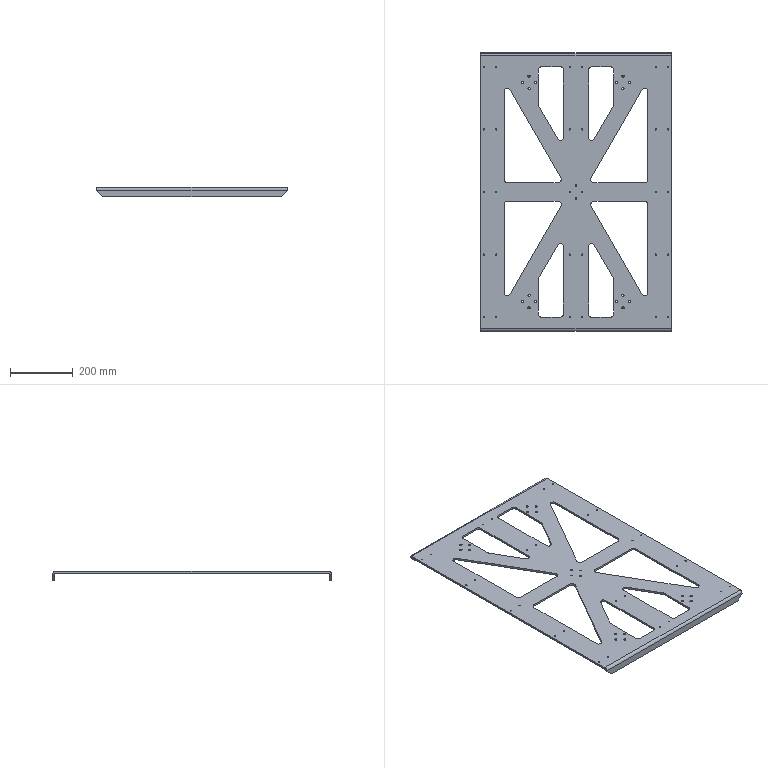Part | STEP file | LIFT.UPPER.PLATE.2.stp | 1 solid | 186 faces | box 610 x 890 x 30 mm | volume 2296280 mm3 | spline 86 | cylinder 80 | plane 20 | commonest cylinder face diameters 4 x30 20 x28 7 x16 6 x4 18 x2